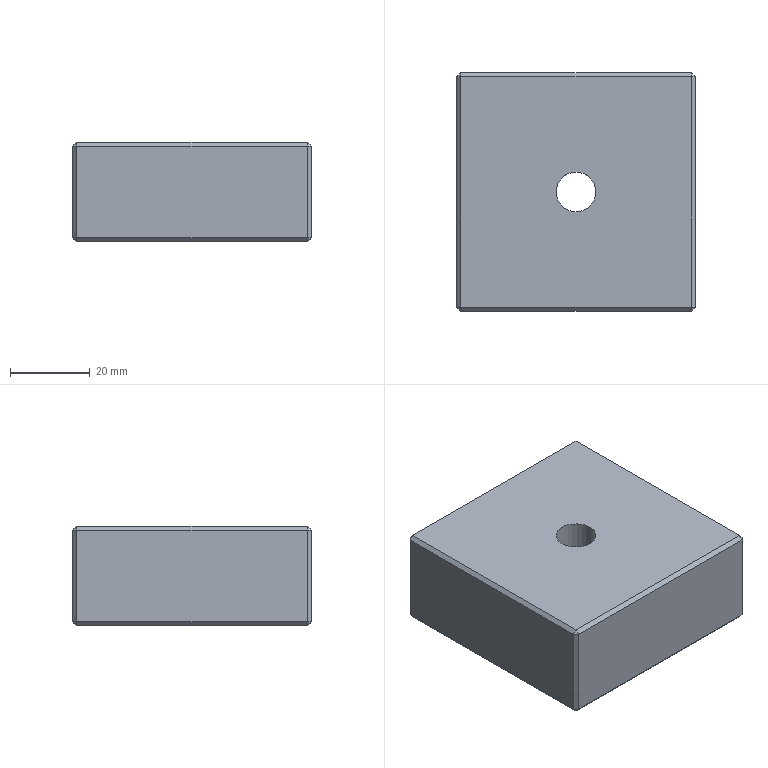Part | SolidWorks | features ICE 2, Chamfer 1, Extrusion 1 | 1 solid | 31 faces | box 60 x 60 x 25 mm | volume 83354 mm3 | plane 27 | cylinder 4 | commonest cylinder face diameters 10 x2 30 x2
STEP:
#1=CARTESIAN_POINT('',(5.,0.,25.));
#2=VERTEX_POINT('',#1);
#3=CARTESIAN_POINT('',(-5.,0.,25.));
#4=VERTEX_POINT('',#3);
#5=CARTESIAN_POINT('',(0.,0.,25.));
#6=DIRECTION('',(0.,0.,-1.));
#7=DIRECTION('',(-1.,0.,0.));
#8=AXIS2_PLACEMENT_3D('',#5,#6,#7);
#9=CIRCLE('',#8,5.);
#10=EDGE_CURVE('',#2,#4,#9,.T.);
#11=ORIENTED_EDGE('',*,*,#10,.F.);
#12=CARTESIAN_POINT('',(5.,0.,7.));
#13=VERTEX_POINT('',#12);
#14=CARTESIAN_POINT('',(5.,0.,25.));
#15=DIRECTION('',(0.,0.,-1.));
#16=VECTOR('',#15,1000.);
#17=LINE('',#14,#16);
#18=EDGE_CURVE('',#2,#13,#17,.T.);
#19=ORIENTED_EDGE('',*,*,#18,.T.);
#20=CARTESIAN_POINT('',(-5.,0.,7.));
#21=VERTEX_POINT('',#20);
#22=CARTESIAN_POINT('',(0.,0.,7.));
#23=DIRECTION('',(0.,0.,-1.));
#24=DIRECTION('',(-1.,0.,0.));
#25=AXIS2_PLACEMENT_3D('',#22,#23,#24);
#26=CIRCLE('',#25,5.);
#27=EDGE_CURVE('',#13,#21,#26,.T.);
#28=ORIENTED_EDGE('',*,*,#27,.T.);
#29=CARTESIAN_POINT('',(-5.,0.,25.));
#30=DIRECTION('',(0.,0.,-1.));
#31=VECTOR('',#30,1000.);
#32=LINE('',#29,#31);
#33=EDGE_CURVE('',#4,#21,#32,.T.);
#34=ORIENTED_EDGE('',*,*,#33,.F.);
#35=EDGE_LOOP('',(#11,#19,#28,#34));
#36=FACE_OUTER_BOUND('',#35,.T.);
#37=CARTESIAN_POINT('',(0.,0.,25.));
#38=DIRECTION('',(0.,0.,-1.));
#39=DIRECTION('',(-1.,0.,0.));
#40=AXIS2_PLACEMENT_3D('',#37,#38,#39);
#41=CYLINDRICAL_SURFACE('',#40,5.);
#42=ADVANCED_FACE('',(#36),#41,.F.);
#43=CARTESIAN_POINT('',(15.,0.,7.));
#44=VERTEX_POINT('',#43);
#45=CARTESIAN_POINT('',(-15.,0.,7.));
#46=VERTEX_POINT('',#45);
#47=CARTESIAN_POINT('',(0.,0.,7.));
#48=DIRECTION('',(0.,0.,-1.));
#49=DIRECTION('',(-1.,0.,0.));
#50=AXIS2_PLACEMENT_3D('',#47,#48,#49);
#51=CIRCLE('',#50,15.);
#52=EDGE_CURVE('',#44,#46,#51,.T.);
#53=ORIENTED_EDGE('',*,*,#52,.F.);
#54=CARTESIAN_POINT('',(15.,0.,0.));
#55=VERTEX_POINT('',#54);
#56=CARTESIAN_POINT('',(15.,0.,7.));
#57=DIRECTION('',(0.,0.,-1.));
#58=VECTOR('',#57,1000.);
#59=LINE('',#56,#58);
#60=EDGE_CURVE('',#44,#55,#59,.T.);
#61=ORIENTED_EDGE('',*,*,#60,.T.);
#62=CARTESIAN_POINT('',(-15.,0.,0.));
#63=VERTEX_POINT('',#62);
#64=CARTESIAN_POINT('',(0.,0.,0.));
#65=DIRECTION('',(0.,0.,-1.));
#66=DIRECTION('',(-1.,0.,0.));
#67=AXIS2_PLACEMENT_3D('',#64,#65,#66);
#68=CIRCLE('',#67,15.);
#69=EDGE_CURVE('',#55,#63,#68,.T.);
#70=ORIENTED_EDGE('',*,*,#69,.T.);
#71=CARTESIAN_POINT('',(-15.,0.,7.));
#72=DIRECTION('',(0.,0.,-1.));
#73=VECTOR('',#72,1000.);
#74=LINE('',#71,#73);
#75=EDGE_CURVE('',#46,#63,#74,.T.);
#76=ORIENTED_EDGE('',*,*,#75,.F.);
#77=EDGE_LOOP('',(#53,#61,#70,#76));
#78=FACE_OUTER_BOUND('',#77,.T.);
#79=CARTESIAN_POINT('',(0.,0.,7.));
#80=DIRECTION('',(0.,0.,-1.));
#81=DIRECTION('',(-1.,0.,0.));
#82=AXIS2_PLACEMENT_3D('',#79,#80,#81);
#83=CYLINDRICAL_SURFACE('',#82,15.);
#84=ADVANCED_FACE('',(#78),#83,.F.);
#85=CARTESIAN_POINT('',(-30.,29.,1.));
#86=VERTEX_POINT('',#85);
#87=CARTESIAN_POINT('',(-30.,-29.,1.));
#88=VERTEX_POINT('',#87);
#89=CARTESIAN_POINT('',(-30.,-30.,1.));
#90=DIRECTION('',(0.,-1.,0.));
#91=VECTOR('',#90,1000.);
#92=LINE('',#89,#91);
#93=EDGE_CURVE('',#86,#88,#92,.T.);
#94=ORIENTED_EDGE('',*,*,#93,.T.);
#95=CARTESIAN_POINT('',(-30.,-29.,24.));
#96=VERTEX_POINT('',#95);
#97=CARTESIAN_POINT('',(-30.,-29.,25.));
#98=DIRECTION('',(0.,0.,1.));
#99=VECTOR('',#98,1000.);
#100=LINE('',#97,#99);
#101=EDGE_CURVE('',#88,#96,#100,.T.);
#102=ORIENTED_EDGE('',*,*,#101,.T.);
#103=CARTESIAN_POINT('',(-30.,29.,24.));
#104=VERTEX_POINT('',#103);
#105=CARTESIAN_POINT('',(-30.,30.,24.));
#106=DIRECTION('',(0.,1.,0.));
#107=VECTOR('',#106,1000.);
#108=LINE('',#105,#107);
#109=EDGE_CURVE('',#96,#104,#108,.T.);
#110=ORIENTED_EDGE('',*,*,#109,.T.);
#111=CARTESIAN_POINT('',(-30.,29.,25.));
#112=DIRECTION('',(0.,0.,-1.));
#113=VECTOR('',#112,1000.);
#114=LINE('',#111,#113);
#115=EDGE_CURVE('',#104,#86,#114,.T.);
#116=ORIENTED_EDGE('',*,*,#115,.T.);
#117=EDGE_LOOP('',(#94,#102,#110,#116));
#118=FACE_OUTER_BOUND('',#117,.T.);
#119=CARTESIAN_POINT('',(-30.,-30.,25.));
#120=DIRECTION('',(-1.,0.,0.));
#121=DIRECTION('',(0.,0.,1.));
#122=AXIS2_PLACEMENT_3D('',#119,#120,#121);
#123=PLANE('',#122);
#124=ADVANCED_FACE('',(#118),#123,.T.);
#125=CARTESIAN_POINT('',(-29.,-30.,1.));
#126=VERTEX_POINT('',#125);
#127=CARTESIAN_POINT('',(29.,-30.,1.));
#128=VERTEX_POINT('',#127);
#129=CARTESIAN_POINT('',(30.,-30.,1.));
#130=DIRECTION('',(1.,0.,0.));
#131=VECTOR('',#130,1000.);
#132=LINE('',#129,#131);
#133=EDGE_CURVE('',#126,#128,#132,.T.);
#134=ORIENTED_EDGE('',*,*,#133,.T.);
#135=CARTESIAN_POINT('',(29.,-30.,24.));
#136=VERTEX_POINT('',#135);
#137=CARTESIAN_POINT('',(29.,-30.,25.));
#138=DIRECTION('',(0.,0.,1.));
#139=VECTOR('',#138,1000.);
#140=LINE('',#137,#139);
#141=EDGE_CURVE('',#128,#136,#140,.T.);
#142=ORIENTED_EDGE('',*,*,#141,.T.);
#143=CARTESIAN_POINT('',(-29.,-30.,24.));
#144=VERTEX_POINT('',#143);
#145=CARTESIAN_POINT('',(-30.,-30.,24.));
#146=DIRECTION('',(-1.,0.,0.));
#147=VECTOR('',#146,1000.);
#148=LINE('',#145,#147);
#149=EDGE_CURVE('',#136,#144,#148,.T.);
#150=ORIENTED_EDGE('',*,*,#149,.T.);
#151=CARTESIAN_POINT('',(-29.,-30.,0.));
#152=DIRECTION('',(0.,0.,-1.));
#153=VECTOR('',#152,1000.);
#154=LINE('',#151,#153);
#155=EDGE_CURVE('',#144,#126,#154,.T.);
#156=ORIENTED_EDGE('',*,*,#155,.T.);
#157=EDGE_LOOP('',(#134,#142,#150,#156));
#158=FACE_OUTER_BOUND('',#157,.T.);
#159=CARTESIAN_POINT('',(-30.,-30.,25.));
#160=DIRECTION('',(0.,1.,0.));
#161=DIRECTION('',(0.,0.,1.));
#162=AXIS2_PLACEMENT_3D('',#159,#160,#161);
#163=PLANE('',#162);
#164=ADVANCED_FACE('',(#158),#163,.F.);
#165=CARTESIAN_POINT('',(30.,-29.,24.));
#166=VERTEX_POINT('',#165);
#167=CARTESIAN_POINT('',(30.,-29.,1.));
#168=VERTEX_POINT('',#167);
#169=CARTESIAN_POINT('',(30.,-29.,25.));
#170=DIRECTION('',(0.,0.,-1.));
#171=VECTOR('',#170,1000.);
#172=LINE('',#169,#171);
#173=EDGE_CURVE('',#166,#168,#172,.T.);
#174=ORIENTED_EDGE('',*,*,#173,.T.);
#175=CARTESIAN_POINT('',(30.,29.,1.));
#176=VERTEX_POINT('',#175);
#177=CARTESIAN_POINT('',(30.,30.,1.));
#178=DIRECTION('',(0.,1.,0.));
#179=VECTOR('',#178,1000.);
#180=LINE('',#177,#179);
#181=EDGE_CURVE('',#168,#176,#180,.T.);
#182=ORIENTED_EDGE('',*,*,#181,.T.);
#183=CARTESIAN_POINT('',(30.,29.,24.));
#184=VERTEX_POINT('',#183);
#185=CARTESIAN_POINT('',(30.,29.,25.));
#186=DIRECTION('',(0.,0.,1.));
#187=VECTOR('',#186,1000.);
#188=LINE('',#185,#187);
#189=EDGE_CURVE('',#176,#184,#188,.T.);
#190=ORIENTED_EDGE('',*,*,#189,.T.);
#191=CARTESIAN_POINT('',(30.,-30.,24.));
#192=DIRECTION('',(0.,-1.,0.));
#193=VECTOR('',#192,1000.);
#194=LINE('',#191,#193);
#195=EDGE_CURVE('',#184,#166,#194,.T.);
#196=ORIENTED_EDGE('',*,*,#195,.T.);
#197=EDGE_LOOP('',(#174,#182,#190,#196));
#198=FACE_OUTER_BOUND('',#197,.T.);
#199=CARTESIAN_POINT('',(30.,-30.,25.));
#200=DIRECTION('',(-1.,0.,0.));
#201=DIRECTION('',(0.,0.,1.));
#202=AXIS2_PLACEMENT_3D('',#199,#200,#201);
#203=PLANE('',#202);
#204=ADVANCED_FACE('',(#198),#203,.F.);
#205=CARTESIAN_POINT('',(-29.,30.,24.));
#206=VERTEX_POINT('',#205);
#207=CARTESIAN_POINT('',(29.,30.,24.));
#208=VERTEX_POINT('',#207);
#209=CARTESIAN_POINT('',(30.,30.,24.));
#210=DIRECTION('',(1.,0.,0.));
#211=VECTOR('',#210,1000.);
#212=LINE('',#209,#211);
#213=EDGE_CURVE('',#206,#208,#212,.T.);
#214=ORIENTED_EDGE('',*,*,#213,.T.);
#215=CARTESIAN_POINT('',(29.,30.,1.));
#216=VERTEX_POINT('',#215);
#217=CARTESIAN_POINT('',(29.,30.,0.));
#218=DIRECTION('',(0.,0.,-1.));
#219=VECTOR('',#218,1000.);
#220=LINE('',#217,#219);
#221=EDGE_CURVE('',#208,#216,#220,.T.);
#222=ORIENTED_EDGE('',*,*,#221,.T.);
#223=CARTESIAN_POINT('',(-29.,30.,1.));
#224=VERTEX_POINT('',#223);
#225=CARTESIAN_POINT('',(-30.,30.,1.));
#226=DIRECTION('',(-1.,0.,0.));
#227=VECTOR('',#226,1000.);
#228=LINE('',#225,#227);
#229=EDGE_CURVE('',#216,#224,#228,.T.);
#230=ORIENTED_EDGE('',*,*,#229,.T.);
#231=CARTESIAN_POINT('',(-29.,30.,25.));
#232=DIRECTION('',(0.,0.,1.));
#233=VECTOR('',#232,1000.);
#234=LINE('',#231,#233);
#235=EDGE_CURVE('',#224,#206,#234,.T.);
#236=ORIENTED_EDGE('',*,*,#235,.T.);
#237=EDGE_LOOP('',(#214,#222,#230,#236));
#238=FACE_OUTER_BOUND('',#237,.T.);
#239=CARTESIAN_POINT('',(-30.,30.,25.));
#240=DIRECTION('',(0.,1.,0.));
#241=DIRECTION('',(0.,0.,1.));
#242=AXIS2_PLACEMENT_3D('',#239,#240,#241);
#243=PLANE('',#242);
#244=ADVANCED_FACE('',(#238),#243,.T.);
#245=CARTESIAN_POINT('',(0.,0.,25.));
#246=DIRECTION('',(0.,0.,-1.));
#247=DIRECTION('',(-1.,0.,0.));
#248=AXIS2_PLACEMENT_3D('',#245,#246,#247);
#249=CIRCLE('',#248,5.);
#250=EDGE_CURVE('',#4,#2,#249,.T.);
#251=ORIENTED_EDGE('',*,*,#250,.T.);
#252=ORIENTED_EDGE('',*,*,#10,.T.);
#253=EDGE_LOOP('',(#251,#252));
#254=FACE_BOUND('',#253,.T.);
#255=CARTESIAN_POINT('',(-29.,29.,25.));
#256=VERTEX_POINT('',#255);
#257=CARTESIAN_POINT('',(-29.,-29.,25.));
#258=VERTEX_POINT('',#257);
#259=CARTESIAN_POINT('',(-29.,-30.,25.));
#260=DIRECTION('',(0.,-1.,0.));
#261=VECTOR('',#260,1000.);
#262=LINE('',#259,#261);
#263=EDGE_CURVE('',#256,#258,#262,.T.);
#264=ORIENTED_EDGE('',*,*,#263,.T.);
#265=CARTESIAN_POINT('',(29.,-29.,25.));
#266=VERTEX_POINT('',#265);
#267=CARTESIAN_POINT('',(0.,-29.,25.));
#268=DIRECTION('',(1.,0.,0.));
#269=VECTOR('',#268,1000.);
#270=LINE('',#267,#269);
#271=EDGE_CURVE('',#258,#266,#270,.T.);
#272=ORIENTED_EDGE('',*,*,#271,.T.);
#273=CARTESIAN_POINT('',(29.,29.,25.));
#274=VERTEX_POINT('',#273);
#275=CARTESIAN_POINT('',(29.,0.,25.));
#276=DIRECTION('',(0.,1.,0.));
#277=VECTOR('',#276,1000.);
#278=LINE('',#275,#277);
#279=EDGE_CURVE('',#266,#274,#278,.T.);
#280=ORIENTED_EDGE('',*,*,#279,.T.);
#281=CARTESIAN_POINT('',(-30.,29.,25.));
#282=DIRECTION('',(-1.,0.,0.));
#283=VECTOR('',#282,1000.);
#284=LINE('',#281,#283);
#285=EDGE_CURVE('',#274,#256,#284,.T.);
#286=ORIENTED_EDGE('',*,*,#285,.T.);
#287=EDGE_LOOP('',(#264,#272,#280,#286));
#288=FACE_OUTER_BOUND('',#287,.T.);
#289=CARTESIAN_POINT('',(0.,0.,25.));
#290=DIRECTION('',(0.,0.,-1.));
#291=DIRECTION('',(-1.,0.,0.));
#292=AXIS2_PLACEMENT_3D('',#289,#290,#291);
#293=PLANE('',#292);
#294=ADVANCED_FACE('',(#254,#288),#293,.F.);
#295=CARTESIAN_POINT('',(0.,0.,0.));
#296=DIRECTION('',(0.,0.,-1.));
#297=DIRECTION('',(-1.,0.,0.));
#298=AXIS2_PLACEMENT_3D('',#295,#296,#297);
#299=CIRCLE('',#298,15.);
#300=EDGE_CURVE('',#63,#55,#299,.T.);
#301=ORIENTED_EDGE('',*,*,#300,.F.);
#302=ORIENTED_EDGE('',*,*,#69,.F.);
#303=EDGE_LOOP('',(#301,#302));
#304=FACE_BOUND('',#303,.T.);
#305=CARTESIAN_POINT('',(-29.,29.,0.));
#306=VERTEX_POINT('',#305);
#307=CARTESIAN_POINT('',(29.,29.,0.));
#308=VERTEX_POINT('',#307);
#309=CARTESIAN_POINT('',(0.,29.,0.));
#310=DIRECTION('',(1.,0.,0.));
#311=VECTOR('',#310,1000.);
#312=LINE('',#309,#311);
#313=EDGE_CURVE('',#306,#308,#312,.T.);
#314=ORIENTED_EDGE('',*,*,#313,.T.);
#315=CARTESIAN_POINT('',(29.,-29.,0.));
#316=VERTEX_POINT('',#315);
#317=CARTESIAN_POINT('',(29.,-30.,0.));
#318=DIRECTION('',(0.,-1.,0.));
#319=VECTOR('',#318,1000.);
#320=LINE('',#317,#319);
#321=EDGE_CURVE('',#308,#316,#320,.T.);
#322=ORIENTED_EDGE('',*,*,#321,.T.);
#323=CARTESIAN_POINT('',(-29.,-29.,0.));
#324=VERTEX_POINT('',#323);
#325=CARTESIAN_POINT('',(-30.,-29.,0.));
#326=DIRECTION('',(-1.,0.,0.));
#327=VECTOR('',#326,1000.);
#328=LINE('',#325,#327);
#329=EDGE_CURVE('',#316,#324,#328,.T.);
#330=ORIENTED_EDGE('',*,*,#329,.T.);
#331=CARTESIAN_POINT('',(-29.,0.,0.));
#332=DIRECTION('',(0.,1.,0.));
#333=VECTOR('',#332,1000.);
#334=LINE('',#331,#333);
#335=EDGE_CURVE('',#324,#306,#334,.T.);
#336=ORIENTED_EDGE('',*,*,#335,.T.);
#337=EDGE_LOOP('',(#314,#322,#330,#336));
#338=FACE_OUTER_BOUND('',#337,.T.);
#339=CARTESIAN_POINT('',(0.,0.,0.));
#340=DIRECTION('',(0.,0.,-1.));
#341=DIRECTION('',(-1.,0.,0.));
#342=AXIS2_PLACEMENT_3D('',#339,#340,#341);
#343=PLANE('',#342);
#344=ADVANCED_FACE('',(#304,#338),#343,.T.);
#345=CARTESIAN_POINT('',(-30.,-29.,24.));
#346=DIRECTION('',(-0.7071,0.,-0.7071));
#347=VECTOR('',#346,1000.);
#348=LINE('',#345,#347);
#349=EDGE_CURVE('',#258,#96,#348,.T.);
#350=ORIENTED_EDGE('',*,*,#349,.F.);
#351=ORIENTED_EDGE('',*,*,#263,.F.);
#352=CARTESIAN_POINT('',(-30.,29.,24.));
#353=DIRECTION('',(0.7071,0.,0.7071));
#354=VECTOR('',#353,1000.);
#355=LINE('',#352,#354);
#356=EDGE_CURVE('',#104,#256,#355,.T.);
#357=ORIENTED_EDGE('',*,*,#356,.F.);
#358=ORIENTED_EDGE('',*,*,#109,.F.);
#359=EDGE_LOOP('',(#350,#351,#357,#358));
#360=FACE_OUTER_BOUND('',#359,.T.);
#361=CARTESIAN_POINT('',(-30.,-30.,24.));
#362=DIRECTION('',(-0.7071,0.,0.7071));
#363=DIRECTION('',(0.,-1.,0.));
#364=AXIS2_PLACEMENT_3D('',#361,#362,#363);
#365=PLANE('',#364);
#366=ADVANCED_FACE('',(#360),#365,.T.);
#367=CARTESIAN_POINT('',(-29.,-29.5,24.5));
#368=DIRECTION('',(0.,-0.7071,-0.7071));
#369=VECTOR('',#368,1000.);
#370=LINE('',#367,#369);
#371=EDGE_CURVE('',#258,#144,#370,.T.);
#372=ORIENTED_EDGE('',*,*,#371,.F.);
#373=ORIENTED_EDGE('',*,*,#349,.T.);
#374=CARTESIAN_POINT('',(-30.,-29.,24.));
#375=DIRECTION('',(-0.7071,0.7071,0.));
#376=VECTOR('',#375,1000.);
#377=LINE('',#374,#376);
#378=EDGE_CURVE('',#144,#96,#377,.T.);
#379=ORIENTED_EDGE('',*,*,#378,.F.);
#380=EDGE_LOOP('',(#372,#373,#379));
#381=FACE_OUTER_BOUND('',#380,.T.);
#382=CARTESIAN_POINT('',(-30.,-29.,24.));
#383=DIRECTION('',(-0.5774,-0.5774,0.5774));
#384=DIRECTION('',(0.7071,0.,0.7071));
#385=AXIS2_PLACEMENT_3D('',#382,#383,#384);
#386=PLANE('',#385);
#387=ADVANCED_FACE('',(#381),#386,.T.);
#388=CARTESIAN_POINT('',(-30.,29.,24.));
#389=DIRECTION('',(0.7071,0.7071,0.));
#390=VECTOR('',#389,1000.);
#391=LINE('',#388,#390);
#392=EDGE_CURVE('',#104,#206,#391,.T.);
#393=ORIENTED_EDGE('',*,*,#392,.F.);
#394=ORIENTED_EDGE('',*,*,#356,.T.);
#395=CARTESIAN_POINT('',(-29.,29.5,24.5));
#396=DIRECTION('',(0.,-0.7071,0.7071));
#397=VECTOR('',#396,1000.);
#398=LINE('',#395,#397);
#399=EDGE_CURVE('',#206,#256,#398,.T.);
#400=ORIENTED_EDGE('',*,*,#399,.F.);
#401=EDGE_LOOP('',(#393,#394,#400));
#402=FACE_OUTER_BOUND('',#401,.T.);
#403=CARTESIAN_POINT('',(-30.,29.,24.));
#404=DIRECTION('',(-0.5774,0.5774,0.5774));
#405=DIRECTION('',(0.7071,0.,0.7071));
#406=AXIS2_PLACEMENT_3D('',#403,#404,#405);
#407=PLANE('',#406);
#408=ADVANCED_FACE('',(#402),#407,.T.);
#409=ORIENTED_EDGE('',*,*,#378,.T.);
#410=ORIENTED_EDGE('',*,*,#101,.F.);
#411=CARTESIAN_POINT('',(-29.5,-29.5,1.));
#412=DIRECTION('',(-0.7071,0.7071,0.));
#413=VECTOR('',#412,1000.);
#414=LINE('',#411,#413);
#415=EDGE_CURVE('',#126,#88,#414,.T.);
#416=ORIENTED_EDGE('',*,*,#415,.F.);
#417=ORIENTED_EDGE('',*,*,#155,.F.);
#418=EDGE_LOOP('',(#409,#410,#416,#417));
#419=FACE_OUTER_BOUND('',#418,.T.);
#420=CARTESIAN_POINT('',(-29.,-30.,25.));
#421=DIRECTION('',(-0.7071,-0.7071,0.));
#422=DIRECTION('',(0.,0.,1.));
#423=AXIS2_PLACEMENT_3D('',#420,#421,#422);
#424=PLANE('',#423);
#425=ADVANCED_FACE('',(#419),#424,.T.);
#426=ORIENTED_EDGE('',*,*,#371,.T.);
#427=ORIENTED_EDGE('',*,*,#149,.F.);
#428=CARTESIAN_POINT('',(29.,-30.,24.));
#429=DIRECTION('',(0.,-0.7071,-0.7071));
#430=VECTOR('',#429,1000.);
#431=LINE('',#428,#430);
#432=EDGE_CURVE('',#266,#136,#431,.T.);
#433=ORIENTED_EDGE('',*,*,#432,.F.);
#434=ORIENTED_EDGE('',*,*,#271,.F.);
#435=EDGE_LOOP('',(#426,#427,#433,#434));
#436=FACE_OUTER_BOUND('',#435,.T.);
#437=CARTESIAN_POINT('',(0.,-29.,25.));
#438=DIRECTION('',(0.,0.7071,-0.7071));
#439=DIRECTION('',(1.,0.,0.));
#440=AXIS2_PLACEMENT_3D('',#437,#438,#439);
#441=PLANE('',#440);
#442=ADVANCED_FACE('',(#436),#441,.F.);
#443=CARTESIAN_POINT('',(29.,29.,25.));
#444=DIRECTION('',(0.7071,0.,-0.7071));
#445=VECTOR('',#444,1000.);
#446=LINE('',#443,#445);
#447=EDGE_CURVE('',#274,#184,#446,.T.);
#448=ORIENTED_EDGE('',*,*,#447,.F.);
#449=ORIENTED_EDGE('',*,*,#279,.F.);
#450=CARTESIAN_POINT('',(29.5,-29.,24.5));
#451=DIRECTION('',(-0.7071,0.,0.7071));
#452=VECTOR('',#451,1000.);
#453=LINE('',#450,#452);
#454=EDGE_CURVE('',#166,#266,#453,.T.);
#455=ORIENTED_EDGE('',*,*,#454,.F.);
#456=ORIENTED_EDGE('',*,*,#195,.F.);
#457=EDGE_LOOP('',(#448,#449,#455,#456));
#458=FACE_OUTER_BOUND('',#457,.T.);
#459=CARTESIAN_POINT('',(29.,0.,25.));
#460=DIRECTION('',(-0.7071,0.,-0.7071));
#461=DIRECTION('',(0.,1.,0.));
#462=AXIS2_PLACEMENT_3D('',#459,#460,#461);
#463=PLANE('',#462);
#464=ADVANCED_FACE('',(#458),#463,.F.);
#465=ORIENTED_EDGE('',*,*,#399,.T.);
#466=ORIENTED_EDGE('',*,*,#285,.F.);
#467=CARTESIAN_POINT('',(29.,29.,25.));
#468=DIRECTION('',(0.,-0.7071,0.7071));
#469=VECTOR('',#468,1000.);
#470=LINE('',#467,#469);
#471=EDGE_CURVE('',#208,#274,#470,.T.);
#472=ORIENTED_EDGE('',*,*,#471,.F.);
#473=ORIENTED_EDGE('',*,*,#213,.F.);
#474=EDGE_LOOP('',(#465,#466,#472,#473));
#475=FACE_OUTER_BOUND('',#474,.T.);
#476=CARTESIAN_POINT('',(-30.,30.,24.));
#477=DIRECTION('',(0.,0.7071,0.7071));
#478=DIRECTION('',(-1.,0.,0.));
#479=AXIS2_PLACEMENT_3D('',#476,#477,#478);
#480=PLANE('',#479);
#481=ADVANCED_FACE('',(#475),#480,.T.);
#482=ORIENTED_EDGE('',*,*,#392,.T.);
#483=ORIENTED_EDGE('',*,*,#235,.F.);
#484=CARTESIAN_POINT('',(-29.5,29.5,1.));
#485=DIRECTION('',(0.7071,0.7071,0.));
#486=VECTOR('',#485,1000.);
#487=LINE('',#484,#486);
#488=EDGE_CURVE('',#86,#224,#487,.T.);
#489=ORIENTED_EDGE('',*,*,#488,.F.);
#490=ORIENTED_EDGE('',*,*,#115,.F.);
#491=EDGE_LOOP('',(#482,#483,#489,#490));
#492=FACE_OUTER_BOUND('',#491,.T.);
#493=CARTESIAN_POINT('',(-30.,29.,25.));
#494=DIRECTION('',(0.7071,-0.7071,0.));
#495=DIRECTION('',(0.,0.,-1.));
#496=AXIS2_PLACEMENT_3D('',#493,#494,#495);
#497=PLANE('',#496);
#498=ADVANCED_FACE('',(#492),#497,.F.);
#499=CARTESIAN_POINT('',(-29.,-29.,0.));
#500=DIRECTION('',(0.7071,0.,-0.7071));
#501=VECTOR('',#500,1000.);
#502=LINE('',#499,#501);
#503=EDGE_CURVE('',#88,#324,#502,.T.);
#504=ORIENTED_EDGE('',*,*,#503,.F.);
#505=ORIENTED_EDGE('',*,*,#93,.F.);
#506=CARTESIAN_POINT('',(-29.,29.,0.));
#507=DIRECTION('',(-0.7071,0.,0.7071));
#508=VECTOR('',#507,1000.);
#509=LINE('',#506,#508);
#510=EDGE_CURVE('',#306,#86,#509,.T.);
#511=ORIENTED_EDGE('',*,*,#510,.F.);
#512=ORIENTED_EDGE('',*,*,#335,.F.);
#513=EDGE_LOOP('',(#504,#505,#511,#512));
#514=FACE_OUTER_BOUND('',#513,.T.);
#515=CARTESIAN_POINT('',(-29.,0.,0.));
#516=DIRECTION('',(0.7071,0.,0.7071));
#517=DIRECTION('',(0.,1.,0.));
#518=AXIS2_PLACEMENT_3D('',#515,#516,#517);
#519=PLANE('',#518);
#520=ADVANCED_FACE('',(#514),#519,.F.);
#521=ORIENTED_EDGE('',*,*,#415,.T.);
#522=ORIENTED_EDGE('',*,*,#503,.T.);
#523=CARTESIAN_POINT('',(-29.,-29.,0.));
#524=DIRECTION('',(0.,0.7071,-0.7071));
#525=VECTOR('',#524,1000.);
#526=LINE('',#523,#525);
#527=EDGE_CURVE('',#126,#324,#526,.T.);
#528=ORIENTED_EDGE('',*,*,#527,.F.);
#529=EDGE_LOOP('',(#521,#522,#528));
#530=FACE_OUTER_BOUND('',#529,.T.);
#531=CARTESIAN_POINT('',(-29.,-29.,0.));
#532=DIRECTION('',(-0.5774,-0.5774,-0.5774));
#533=DIRECTION('',(-0.7071,0.,0.7071));
#534=AXIS2_PLACEMENT_3D('',#531,#532,#533);
#535=PLANE('',#534);
#536=ADVANCED_FACE('',(#530),#535,.T.);
#537=ORIENTED_EDGE('',*,*,#454,.T.);
#538=ORIENTED_EDGE('',*,*,#432,.T.);
#539=CARTESIAN_POINT('',(29.,-30.,24.));
#540=DIRECTION('',(-0.7071,-0.7071,0.));
#541=VECTOR('',#540,1000.);
#542=LINE('',#539,#541);
#543=EDGE_CURVE('',#166,#136,#542,.T.);
#544=ORIENTED_EDGE('',*,*,#543,.F.);
#545=EDGE_LOOP('',(#537,#538,#544));
#546=FACE_OUTER_BOUND('',#545,.T.);
#547=CARTESIAN_POINT('',(29.,-30.,24.));
#548=DIRECTION('',(0.5774,-0.5774,0.5774));
#549=DIRECTION('',(0.7071,0.,-0.7071));
#550=AXIS2_PLACEMENT_3D('',#547,#548,#549);
#551=PLANE('',#550);
#552=ADVANCED_FACE('',(#546),#551,.T.);
#553=ORIENTED_EDGE('',*,*,#471,.T.);
#554=ORIENTED_EDGE('',*,*,#447,.T.);
#555=CARTESIAN_POINT('',(29.5,29.5,24.));
#556=DIRECTION('',(0.7071,-0.7071,0.));
#557=VECTOR('',#556,1000.);
#558=LINE('',#555,#557);
#559=EDGE_CURVE('',#208,#184,#558,.T.);
#560=ORIENTED_EDGE('',*,*,#559,.F.);
#561=EDGE_LOOP('',(#553,#554,#560));
#562=FACE_OUTER_BOUND('',#561,.T.);
#563=CARTESIAN_POINT('',(29.,29.,25.));
#564=DIRECTION('',(0.5774,0.5774,0.5774));
#565=DIRECTION('',(0.7071,0.,-0.7071));
#566=AXIS2_PLACEMENT_3D('',#563,#564,#565);
#567=PLANE('',#566);
#568=ADVANCED_FACE('',(#562),#567,.T.);
#569=ORIENTED_EDGE('',*,*,#510,.T.);
#570=ORIENTED_EDGE('',*,*,#488,.T.);
#571=CARTESIAN_POINT('',(-29.,29.,0.));
#572=DIRECTION('',(0.,0.7071,0.7071));
#573=VECTOR('',#572,1000.);
#574=LINE('',#571,#573);
#575=EDGE_CURVE('',#306,#224,#574,.T.);
#576=ORIENTED_EDGE('',*,*,#575,.F.);
#577=EDGE_LOOP('',(#569,#570,#576));
#578=FACE_OUTER_BOUND('',#577,.T.);
#579=CARTESIAN_POINT('',(-29.,29.,0.));
#580=DIRECTION('',(-0.5774,0.5774,-0.5774));
#581=DIRECTION('',(-0.7071,0.,0.7071));
#582=AXIS2_PLACEMENT_3D('',#579,#580,#581);
#583=PLANE('',#582);
#584=ADVANCED_FACE('',(#578),#583,.T.);
#585=ORIENTED_EDGE('',*,*,#527,.T.);
#586=ORIENTED_EDGE('',*,*,#329,.F.);
#587=CARTESIAN_POINT('',(29.,-29.,0.));
#588=DIRECTION('',(0.,0.7071,-0.7071));
#589=VECTOR('',#588,1000.);
#590=LINE('',#587,#589);
#591=EDGE_CURVE('',#128,#316,#590,.T.);
#592=ORIENTED_EDGE('',*,*,#591,.F.);
#593=ORIENTED_EDGE('',*,*,#133,.F.);
#594=EDGE_LOOP('',(#585,#586,#592,#593));
#595=FACE_OUTER_BOUND('',#594,.T.);
#596=CARTESIAN_POINT('',(-30.,-30.,1.));
#597=DIRECTION('',(0.,-0.7071,-0.7071));
#598=DIRECTION('',(-1.,0.,0.));
#599=AXIS2_PLACEMENT_3D('',#596,#597,#598);
#600=PLANE('',#599);
#601=ADVANCED_FACE('',(#595),#600,.T.);
#602=ORIENTED_EDGE('',*,*,#543,.T.);
#603=ORIENTED_EDGE('',*,*,#141,.F.);
#604=CARTESIAN_POINT('',(29.5,-29.5,1.));
#605=DIRECTION('',(-0.7071,-0.7071,0.));
#606=VECTOR('',#605,1000.);
#607=LINE('',#604,#606);
#608=EDGE_CURVE('',#168,#128,#607,.T.);
#609=ORIENTED_EDGE('',*,*,#608,.F.);
#610=ORIENTED_EDGE('',*,*,#173,.F.);
#611=EDGE_LOOP('',(#602,#603,#609,#610));
#612=FACE_OUTER_BOUND('',#611,.T.);
#613=CARTESIAN_POINT('',(30.,-29.,25.));
#614=DIRECTION('',(-0.7071,0.7071,0.));
#615=DIRECTION('',(0.,0.,-1.));
#616=AXIS2_PLACEMENT_3D('',#613,#614,#615);
#617=PLANE('',#616);
#618=ADVANCED_FACE('',(#612),#617,.F.);
#619=ORIENTED_EDGE('',*,*,#559,.T.);
#620=ORIENTED_EDGE('',*,*,#189,.F.);
#621=CARTESIAN_POINT('',(30.,29.,1.));
#622=DIRECTION('',(0.7071,-0.7071,0.));
#623=VECTOR('',#622,1000.);
#624=LINE('',#621,#623);
#625=EDGE_CURVE('',#216,#176,#624,.T.);
#626=ORIENTED_EDGE('',*,*,#625,.F.);
#627=ORIENTED_EDGE('',*,*,#221,.F.);
#628=EDGE_LOOP('',(#619,#620,#626,#627));
#629=FACE_OUTER_BOUND('',#628,.T.);
#630=CARTESIAN_POINT('',(29.,30.,25.));
#631=DIRECTION('',(0.7071,0.7071,0.));
#632=DIRECTION('',(0.,0.,1.));
#633=AXIS2_PLACEMENT_3D('',#630,#631,#632);
#634=PLANE('',#633);
#635=ADVANCED_FACE('',(#629),#634,.T.);
#636=ORIENTED_EDGE('',*,*,#575,.T.);
#637=ORIENTED_EDGE('',*,*,#229,.F.);
#638=CARTESIAN_POINT('',(29.,29.5,0.5));
#639=DIRECTION('',(0.,0.7071,0.7071));
#640=VECTOR('',#639,1000.);
#641=LINE('',#638,#640);
#642=EDGE_CURVE('',#308,#216,#641,.T.);
#643=ORIENTED_EDGE('',*,*,#642,.F.);
#644=ORIENTED_EDGE('',*,*,#313,.F.);
#645=EDGE_LOOP('',(#636,#637,#643,#644));
#646=FACE_OUTER_BOUND('',#645,.T.);
#647=CARTESIAN_POINT('',(0.,29.,0.));
#648=DIRECTION('',(0.,-0.7071,0.7071));
#649=DIRECTION('',(1.,0.,0.));
#650=AXIS2_PLACEMENT_3D('',#647,#648,#649);
#651=PLANE('',#650);
#652=ADVANCED_FACE('',(#646),#651,.F.);
#653=ORIENTED_EDGE('',*,*,#608,.T.);
#654=ORIENTED_EDGE('',*,*,#591,.T.);
#655=CARTESIAN_POINT('',(29.,-29.,0.));
#656=DIRECTION('',(-0.7071,0.,-0.7071));
#657=VECTOR('',#656,1000.);
#658=LINE('',#655,#657);
#659=EDGE_CURVE('',#168,#316,#658,.T.);
#660=ORIENTED_EDGE('',*,*,#659,.F.);
#661=EDGE_LOOP('',(#653,#654,#660));
#662=FACE_OUTER_BOUND('',#661,.T.);
#663=CARTESIAN_POINT('',(29.,-29.,0.));
#664=DIRECTION('',(0.5774,-0.5774,-0.5774));
#665=DIRECTION('',(-0.7071,0.,-0.7071));
#666=AXIS2_PLACEMENT_3D('',#663,#664,#665);
#667=PLANE('',#666);
#668=ADVANCED_FACE('',(#662),#667,.T.);
#669=ORIENTED_EDGE('',*,*,#642,.T.);
#670=ORIENTED_EDGE('',*,*,#625,.T.);
#671=CARTESIAN_POINT('',(30.,29.,1.));
#672=DIRECTION('',(0.7071,0.,0.7071));
#673=VECTOR('',#672,1000.);
#674=LINE('',#671,#673);
#675=EDGE_CURVE('',#308,#176,#674,.T.);
#676=ORIENTED_EDGE('',*,*,#675,.F.);
#677=EDGE_LOOP('',(#669,#670,#676));
#678=FACE_OUTER_BOUND('',#677,.T.);
#679=CARTESIAN_POINT('',(30.,29.,1.));
#680=DIRECTION('',(0.5774,0.5774,-0.5774));
#681=DIRECTION('',(-0.7071,0.,-0.7071));
#682=AXIS2_PLACEMENT_3D('',#679,#680,#681);
#683=PLANE('',#682);
#684=ADVANCED_FACE('',(#678),#683,.T.);
#685=ORIENTED_EDGE('',*,*,#659,.T.);
#686=ORIENTED_EDGE('',*,*,#321,.F.);
#687=ORIENTED_EDGE('',*,*,#675,.T.);
#688=ORIENTED_EDGE('',*,*,#181,.F.);
#689=EDGE_LOOP('',(#685,#686,#687,#688));
#690=FACE_OUTER_BOUND('',#689,.T.);
#691=CARTESIAN_POINT('',(30.,-30.,1.));
#692=DIRECTION('',(0.7071,0.,-0.7071));
#693=DIRECTION('',(0.,-1.,0.));
#694=AXIS2_PLACEMENT_3D('',#691,#692,#693);
#695=PLANE('',#694);
#696=ADVANCED_FACE('',(#690),#695,.T.);
#697=ORIENTED_EDGE('',*,*,#60,.F.);
#698=CARTESIAN_POINT('',(0.,0.,7.));
#699=DIRECTION('',(0.,0.,-1.));
#700=DIRECTION('',(-1.,0.,0.));
#701=AXIS2_PLACEMENT_3D('',#698,#699,#700);
#702=CIRCLE('',#701,15.);
#703=EDGE_CURVE('',#46,#44,#702,.T.);
#704=ORIENTED_EDGE('',*,*,#703,.F.);
#705=ORIENTED_EDGE('',*,*,#75,.T.);
#706=ORIENTED_EDGE('',*,*,#300,.T.);
#707=EDGE_LOOP('',(#697,#704,#705,#706));
#708=FACE_OUTER_BOUND('',#707,.T.);
#709=CARTESIAN_POINT('',(0.,0.,7.));
#710=DIRECTION('',(0.,0.,-1.));
#711=DIRECTION('',(-1.,0.,0.));
#712=AXIS2_PLACEMENT_3D('',#709,#710,#711);
#713=CYLINDRICAL_SURFACE('',#712,15.);
#714=ADVANCED_FACE('',(#708),#713,.F.);
#715=CARTESIAN_POINT('',(0.,0.,7.));
#716=DIRECTION('',(0.,0.,-1.));
#717=DIRECTION('',(-1.,0.,0.));
#718=AXIS2_PLACEMENT_3D('',#715,#716,#717);
#719=CIRCLE('',#718,5.);
#720=EDGE_CURVE('',#21,#13,#719,.T.);
#721=ORIENTED_EDGE('',*,*,#720,.F.);
#722=ORIENTED_EDGE('',*,*,#27,.F.);
#723=EDGE_LOOP('',(#721,#722));
#724=FACE_BOUND('',#723,.T.);
#725=ORIENTED_EDGE('',*,*,#703,.T.);
#726=ORIENTED_EDGE('',*,*,#52,.T.);
#727=EDGE_LOOP('',(#725,#726));
#728=FACE_OUTER_BOUND('',#727,.T.);
#729=CARTESIAN_POINT('',(0.,0.,7.));
#730=DIRECTION('',(0.,0.,-1.));
#731=DIRECTION('',(-1.,0.,0.));
#732=AXIS2_PLACEMENT_3D('',#729,#730,#731);
#733=PLANE('',#732);
#734=ADVANCED_FACE('',(#724,#728),#733,.T.);
#735=ORIENTED_EDGE('',*,*,#18,.F.);
#736=ORIENTED_EDGE('',*,*,#250,.F.);
#737=ORIENTED_EDGE('',*,*,#33,.T.);
#738=ORIENTED_EDGE('',*,*,#720,.T.);
#739=EDGE_LOOP('',(#735,#736,#737,#738));
#740=FACE_OUTER_BOUND('',#739,.T.);
#741=CARTESIAN_POINT('',(0.,0.,25.));
#742=DIRECTION('',(0.,0.,-1.));
#743=DIRECTION('',(-1.,0.,0.));
#744=AXIS2_PLACEMENT_3D('',#741,#742,#743);
#745=CYLINDRICAL_SURFACE('',#744,5.);
#746=ADVANCED_FACE('',(#740),#745,.F.);
#747=CLOSED_SHELL('',(#42,#84,#124,#164,#204,#244,#294,#344,#366,#387,#408,#425,#442,#464,#481,#498,#520,#536,#552,#568,#584,#601,#618,#635,#652,#668,#684,#696,#714,#734,#746));
#748=MANIFOLD_SOLID_BREP('',#747);
#749=CARTESIAN_POINT('',(0.,0.,0.));
#750=DIRECTION('',(0.,0.,1.));
#751=DIRECTION('',(1.,0.,0.));
#752=AXIS2_PLACEMENT_3D('',#749,#750,#751);
#753=(LENGTH_UNIT()NAMED_UNIT(*)SI_UNIT(.MILLI.,.METRE.));
#754=UNCERTAINTY_MEASURE_WITH_UNIT(LENGTH_MEASURE(0.00001),#753,'','');
#755=(NAMED_UNIT(*)PLANE_ANGLE_UNIT()SI_UNIT($,.RADIAN.));
#756=(NAMED_UNIT(*)SI_UNIT($,.STERADIAN.)SOLID_ANGLE_UNIT());
#757=(GEOMETRIC_REPRESENTATION_CONTEXT(3)GLOBAL_UNCERTAINTY_ASSIGNED_CONTEXT((#754))GLOBAL_UNIT_ASSIGNED_CONTEXT((#753,#755,#756))REPRESENTATION_CONTEXT('',''));
#758=ADVANCED_BREP_SHAPE_REPRESENTATION('',(#748,#752),#757);